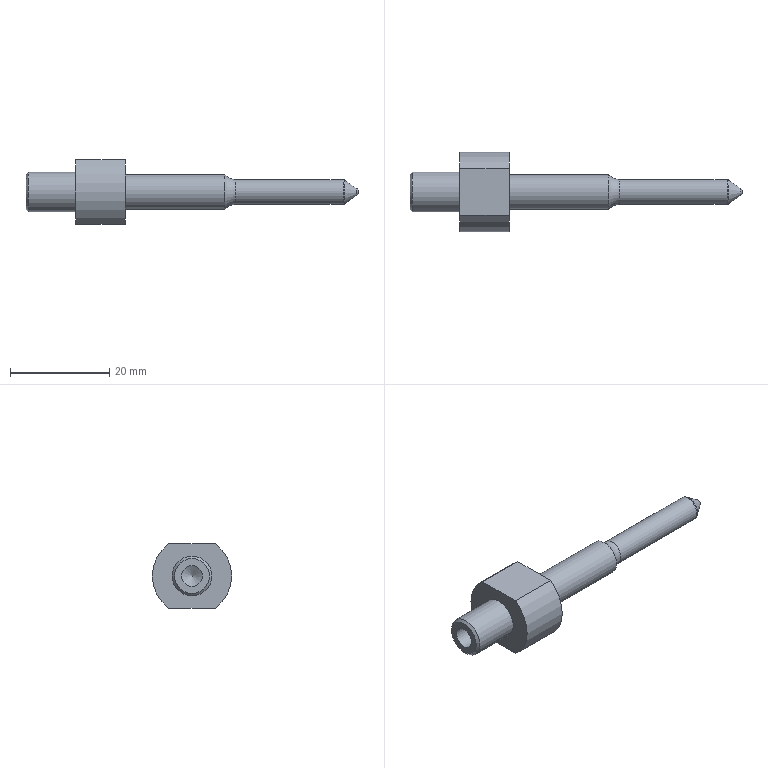Part | NX | features BREP 1 | 1 solid | 18 faces | box 66.856 x 16 x 13 mm | volume 3418 mm3 | cylinder 6 | plane 6 | torus 3 | cone 3 | commonest cylinder face diameters 16 x2 4.2 x1 5 x1 7 x1 8 x1
STEP:
#1=CARTESIAN_POINT('',(-13.428,0.,3.5));
#2=VERTEX_POINT('',#1);
#3=CARTESIAN_POINT('',(-13.428,0.,0.));
#4=DIRECTION('',(1.,0.,0.));
#5=DIRECTION('',(0.,0.,1.));
#6=AXIS2_PLACEMENT_3D('',#3,#4,#5);
#7=CIRCLE('',#6,3.5);
#8=EDGE_CURVE('',#2,#2,#7,.T.);
#9=ORIENTED_EDGE('',*,*,#8,.T.);
#10=EDGE_LOOP('',(#9));
#11=FACE_BOUND('',#10,.T.);
#12=CARTESIAN_POINT('',(6.572,0.,3.5));
#13=VERTEX_POINT('',#12);
#14=CARTESIAN_POINT('',(6.572,0.,0.));
#15=DIRECTION('',(-1.,0.,0.));
#16=DIRECTION('',(0.,0.,1.));
#17=AXIS2_PLACEMENT_3D('',#14,#15,#16);
#18=CIRCLE('',#17,3.5);
#19=EDGE_CURVE('',#13,#13,#18,.T.);
#20=ORIENTED_EDGE('',*,*,#19,.T.);
#21=EDGE_LOOP('',(#20));
#22=FACE_BOUND('',#21,.T.);
#23=CARTESIAN_POINT('',(6.572,0.,0.));
#24=DIRECTION('',(-1.,0.,0.));
#25=DIRECTION('',(0.,0.,-1.));
#26=AXIS2_PLACEMENT_3D('',#23,#24,#25);
#27=CYLINDRICAL_SURFACE('',#26,3.5);
#28=ADVANCED_FACE('',(#11,#22),#27,.T.);
#29=CARTESIAN_POINT('',(-13.428,4.664,-6.5));
#30=VERTEX_POINT('',#29);
#31=CARTESIAN_POINT('',(-13.428,-4.664,-6.5));
#32=VERTEX_POINT('',#31);
#33=CARTESIAN_POINT('',(-13.428,2.5,-6.5));
#34=DIRECTION('',(0.,-1.,0.));
#35=VECTOR('',#34,1000.);
#36=LINE('',#33,#35);
#37=EDGE_CURVE('',#30,#32,#36,.T.);
#38=ORIENTED_EDGE('',*,*,#37,.F.);
#39=CARTESIAN_POINT('',(-13.428,4.664,6.5));
#40=VERTEX_POINT('',#39);
#41=CARTESIAN_POINT('',(-13.428,0.,0.));
#42=DIRECTION('',(-1.,0.,0.));
#43=DIRECTION('',(0.,0.,1.));
#44=AXIS2_PLACEMENT_3D('',#41,#42,#43);
#45=CIRCLE('',#44,8.);
#46=EDGE_CURVE('',#40,#30,#45,.T.);
#47=ORIENTED_EDGE('',*,*,#46,.F.);
#48=CARTESIAN_POINT('',(-13.428,-4.664,6.5));
#49=VERTEX_POINT('',#48);
#50=CARTESIAN_POINT('',(-13.428,2.5,6.5));
#51=DIRECTION('',(0.,1.,0.));
#52=VECTOR('',#51,1000.);
#53=LINE('',#50,#52);
#54=EDGE_CURVE('',#49,#40,#53,.T.);
#55=ORIENTED_EDGE('',*,*,#54,.F.);
#56=CARTESIAN_POINT('',(-13.428,0.,0.));
#57=DIRECTION('',(-1.,0.,0.));
#58=DIRECTION('',(0.,0.,1.));
#59=AXIS2_PLACEMENT_3D('',#56,#57,#58);
#60=CIRCLE('',#59,8.);
#61=EDGE_CURVE('',#32,#49,#60,.T.);
#62=ORIENTED_EDGE('',*,*,#61,.F.);
#63=EDGE_LOOP('',(#38,#47,#55,#62));
#64=FACE_BOUND('',#63,.T.);
#65=ORIENTED_EDGE('',*,*,#8,.F.);
#66=EDGE_LOOP('',(#65));
#67=FACE_BOUND('',#66,.T.);
#68=CARTESIAN_POINT('',(-13.428,2.5,0.));
#69=DIRECTION('',(-1.,0.,0.));
#70=DIRECTION('',(0.,0.,-1.));
#71=AXIS2_PLACEMENT_3D('',#68,#69,#70);
#72=PLANE('',#71);
#73=ADVANCED_FACE('',(#64,#67),#72,.F.);
#74=ORIENTED_EDGE('',*,*,#19,.F.);
#75=EDGE_LOOP('',(#74));
#76=FACE_BOUND('',#75,.T.);
#77=CARTESIAN_POINT('',(8.808,0.,2.5));
#78=VERTEX_POINT('',#77);
#79=CARTESIAN_POINT('',(8.808,0.,0.));
#80=DIRECTION('',(1.,0.,0.));
#81=DIRECTION('',(0.,0.,1.));
#82=AXIS2_PLACEMENT_3D('',#79,#80,#81);
#83=CIRCLE('',#82,2.5);
#84=EDGE_CURVE('',#78,#78,#83,.T.);
#85=ORIENTED_EDGE('',*,*,#84,.F.);
#86=EDGE_LOOP('',(#85));
#87=FACE_BOUND('',#86,.T.);
#88=CARTESIAN_POINT('',(8.808,0.,0.));
#89=DIRECTION('',(-1.,0.,0.));
#90=DIRECTION('',(0.,0.,1.));
#91=AXIS2_PLACEMENT_3D('',#88,#89,#90);
#92=TOROIDAL_SURFACE('',#91,5.5,3.);
#93=ADVANCED_FACE('',(#76,#87),#92,.F.);
#94=ORIENTED_EDGE('',*,*,#61,.T.);
#95=CARTESIAN_POINT('',(-23.428,-4.664,6.5));
#96=VERTEX_POINT('',#95);
#97=CARTESIAN_POINT('',(-33.428,-4.664,6.5));
#98=DIRECTION('',(-1.,0.,0.));
#99=VECTOR('',#98,1000.);
#100=LINE('',#97,#99);
#101=EDGE_CURVE('',#49,#96,#100,.T.);
#102=ORIENTED_EDGE('',*,*,#101,.T.);
#103=CARTESIAN_POINT('',(-23.428,-4.664,-6.5));
#104=VERTEX_POINT('',#103);
#105=CARTESIAN_POINT('',(-23.428,0.,0.));
#106=DIRECTION('',(1.,0.,0.));
#107=DIRECTION('',(0.,0.,1.));
#108=AXIS2_PLACEMENT_3D('',#105,#106,#107);
#109=CIRCLE('',#108,8.);
#110=EDGE_CURVE('',#96,#104,#109,.T.);
#111=ORIENTED_EDGE('',*,*,#110,.T.);
#112=CARTESIAN_POINT('',(-33.428,-4.664,-6.5));
#113=DIRECTION('',(1.,0.,0.));
#114=VECTOR('',#113,1000.);
#115=LINE('',#112,#114);
#116=EDGE_CURVE('',#104,#32,#115,.T.);
#117=ORIENTED_EDGE('',*,*,#116,.T.);
#118=EDGE_LOOP('',(#94,#102,#111,#117));
#119=FACE_BOUND('',#118,.T.);
#120=CARTESIAN_POINT('',(-33.428,0.,0.));
#121=DIRECTION('',(-1.,0.,0.));
#122=DIRECTION('',(0.,0.,-1.));
#123=AXIS2_PLACEMENT_3D('',#120,#121,#122);
#124=CYLINDRICAL_SURFACE('',#123,8.);
#125=ADVANCED_FACE('',(#119),#124,.T.);
#126=ORIENTED_EDGE('',*,*,#116,.F.);
#127=CARTESIAN_POINT('',(-23.428,4.664,-6.5));
#128=VERTEX_POINT('',#127);
#129=CARTESIAN_POINT('',(-23.428,6.928,-6.5));
#130=DIRECTION('',(0.,-1.,0.));
#131=VECTOR('',#130,1000.);
#132=LINE('',#129,#131);
#133=EDGE_CURVE('',#128,#104,#132,.T.);
#134=ORIENTED_EDGE('',*,*,#133,.F.);
#135=CARTESIAN_POINT('',(33.428,4.664,-6.5));
#136=DIRECTION('',(-1.,0.,0.));
#137=VECTOR('',#136,1000.);
#138=LINE('',#135,#137);
#139=EDGE_CURVE('',#30,#128,#138,.T.);
#140=ORIENTED_EDGE('',*,*,#139,.F.);
#141=ORIENTED_EDGE('',*,*,#37,.T.);
#142=EDGE_LOOP('',(#126,#134,#140,#141));
#143=FACE_BOUND('',#142,.T.);
#144=CARTESIAN_POINT('',(33.428,6.928,-6.5));
#145=DIRECTION('',(0.,0.,1.));
#146=DIRECTION('',(-1.,0.,0.));
#147=AXIS2_PLACEMENT_3D('',#144,#145,#146);
#148=PLANE('',#147);
#149=ADVANCED_FACE('',(#143),#148,.F.);
#150=CARTESIAN_POINT('',(-23.428,4.664,6.5));
#151=VERTEX_POINT('',#150);
#152=CARTESIAN_POINT('',(-23.428,0.,0.));
#153=DIRECTION('',(1.,0.,0.));
#154=DIRECTION('',(0.,0.,1.));
#155=AXIS2_PLACEMENT_3D('',#152,#153,#154);
#156=CIRCLE('',#155,8.);
#157=EDGE_CURVE('',#128,#151,#156,.T.);
#158=ORIENTED_EDGE('',*,*,#157,.T.);
#159=CARTESIAN_POINT('',(-33.428,4.664,6.5));
#160=DIRECTION('',(1.,0.,0.));
#161=VECTOR('',#160,1000.);
#162=LINE('',#159,#161);
#163=EDGE_CURVE('',#151,#40,#162,.T.);
#164=ORIENTED_EDGE('',*,*,#163,.T.);
#165=ORIENTED_EDGE('',*,*,#46,.T.);
#166=ORIENTED_EDGE('',*,*,#139,.T.);
#167=EDGE_LOOP('',(#158,#164,#165,#166));
#168=FACE_BOUND('',#167,.T.);
#169=CARTESIAN_POINT('',(-33.428,0.,0.));
#170=DIRECTION('',(-1.,0.,0.));
#171=DIRECTION('',(0.,0.,-1.));
#172=AXIS2_PLACEMENT_3D('',#169,#170,#171);
#173=CYLINDRICAL_SURFACE('',#172,8.);
#174=ADVANCED_FACE('',(#168),#173,.T.);
#175=ORIENTED_EDGE('',*,*,#163,.F.);
#176=CARTESIAN_POINT('',(-23.428,7.156,6.5));
#177=DIRECTION('',(0.,1.,0.));
#178=VECTOR('',#177,1000.);
#179=LINE('',#176,#178);
#180=EDGE_CURVE('',#96,#151,#179,.T.);
#181=ORIENTED_EDGE('',*,*,#180,.F.);
#182=ORIENTED_EDGE('',*,*,#101,.F.);
#183=ORIENTED_EDGE('',*,*,#54,.T.);
#184=EDGE_LOOP('',(#175,#181,#182,#183));
#185=FACE_BOUND('',#184,.T.);
#186=CARTESIAN_POINT('',(33.428,7.156,6.5));
#187=DIRECTION('',(0.,0.,-1.));
#188=DIRECTION('',(1.,0.,0.));
#189=AXIS2_PLACEMENT_3D('',#186,#187,#188);
#190=PLANE('',#189);
#191=ADVANCED_FACE('',(#185),#190,.F.);
#192=ORIENTED_EDGE('',*,*,#84,.T.);
#193=EDGE_LOOP('',(#192));
#194=FACE_BOUND('',#193,.T.);
#195=CARTESIAN_POINT('',(30.414,0.,2.5));
#196=VERTEX_POINT('',#195);
#197=CARTESIAN_POINT('',(30.414,0.,0.));
#198=DIRECTION('',(-1.,0.,0.));
#199=DIRECTION('',(0.,0.,1.));
#200=AXIS2_PLACEMENT_3D('',#197,#198,#199);
#201=CIRCLE('',#200,2.5);
#202=EDGE_CURVE('',#196,#196,#201,.T.);
#203=ORIENTED_EDGE('',*,*,#202,.T.);
#204=EDGE_LOOP('',(#203));
#205=FACE_BOUND('',#204,.T.);
#206=CARTESIAN_POINT('',(-33.428,0.,0.));
#207=DIRECTION('',(-1.,0.,0.));
#208=DIRECTION('',(0.,0.,-1.));
#209=AXIS2_PLACEMENT_3D('',#206,#207,#208);
#210=CYLINDRICAL_SURFACE('',#209,2.5);
#211=ADVANCED_FACE('',(#194,#205),#210,.T.);
#212=ORIENTED_EDGE('',*,*,#133,.T.);
#213=ORIENTED_EDGE('',*,*,#110,.F.);
#214=ORIENTED_EDGE('',*,*,#180,.T.);
#215=ORIENTED_EDGE('',*,*,#157,.F.);
#216=EDGE_LOOP('',(#212,#213,#214,#215));
#217=FACE_BOUND('',#216,.T.);
#218=CARTESIAN_POINT('',(-23.428,0.,4.));
#219=VERTEX_POINT('',#218);
#220=CARTESIAN_POINT('',(-23.428,0.,0.));
#221=DIRECTION('',(-1.,0.,0.));
#222=DIRECTION('',(0.,0.,1.));
#223=AXIS2_PLACEMENT_3D('',#220,#221,#222);
#224=CIRCLE('',#223,4.);
#225=EDGE_CURVE('',#219,#219,#224,.T.);
#226=ORIENTED_EDGE('',*,*,#225,.F.);
#227=EDGE_LOOP('',(#226));
#228=FACE_BOUND('',#227,.T.);
#229=CARTESIAN_POINT('',(-23.428,8.,0.));
#230=DIRECTION('',(1.,0.,0.));
#231=DIRECTION('',(0.,0.,1.));
#232=AXIS2_PLACEMENT_3D('',#229,#230,#231);
#233=PLANE('',#232);
#234=ADVANCED_FACE('',(#217,#228),#233,.F.);
#235=CARTESIAN_POINT('',(30.701,0.,-2.41));
#236=VERTEX_POINT('',#235);
#237=CARTESIAN_POINT('',(30.701,0.,0.));
#238=DIRECTION('',(-1.,0.,0.));
#239=DIRECTION('',(0.,0.,-1.));
#240=AXIS2_PLACEMENT_3D('',#237,#238,#239);
#241=CIRCLE('',#240,2.41);
#242=EDGE_CURVE('',#236,#236,#241,.T.);
#243=ORIENTED_EDGE('',*,*,#242,.T.);
#244=EDGE_LOOP('',(#243));
#245=FACE_BOUND('',#244,.T.);
#246=ORIENTED_EDGE('',*,*,#202,.F.);
#247=EDGE_LOOP('',(#246));
#248=FACE_BOUND('',#247,.T.);
#249=CARTESIAN_POINT('',(30.414,0.,0.));
#250=DIRECTION('',(1.,0.,0.));
#251=DIRECTION('',(0.,0.,-1.));
#252=AXIS2_PLACEMENT_3D('',#249,#250,#251);
#253=TOROIDAL_SURFACE('',#252,2.,0.5);
#254=ADVANCED_FACE('',(#245,#248),#253,.T.);
#255=CARTESIAN_POINT('',(-32.928,0.,4.));
#256=VERTEX_POINT('',#255);
#257=CARTESIAN_POINT('',(-32.928,0.,0.));
#258=DIRECTION('',(1.,0.,0.));
#259=DIRECTION('',(0.,0.,1.));
#260=AXIS2_PLACEMENT_3D('',#257,#258,#259);
#261=CIRCLE('',#260,4.);
#262=EDGE_CURVE('',#256,#256,#261,.T.);
#263=ORIENTED_EDGE('',*,*,#262,.T.);
#264=EDGE_LOOP('',(#263));
#265=FACE_BOUND('',#264,.T.);
#266=ORIENTED_EDGE('',*,*,#225,.T.);
#267=EDGE_LOOP('',(#266));
#268=FACE_BOUND('',#267,.T.);
#269=CARTESIAN_POINT('',(-33.428,0.,0.));
#270=DIRECTION('',(-1.,0.,0.));
#271=DIRECTION('',(0.,0.,-1.));
#272=AXIS2_PLACEMENT_3D('',#269,#270,#271);
#273=CYLINDRICAL_SURFACE('',#272,4.);
#274=ADVANCED_FACE('',(#265,#268),#273,.T.);
#275=ORIENTED_EDGE('',*,*,#242,.F.);
#276=EDGE_LOOP('',(#275));
#277=FACE_BOUND('',#276,.T.);
#278=CARTESIAN_POINT('',(33.215,0.,0.6493));
#279=VERTEX_POINT('',#278);
#280=CARTESIAN_POINT('',(33.215,0.,0.));
#281=DIRECTION('',(-1.,0.,0.));
#282=DIRECTION('',(0.,0.,1.));
#283=AXIS2_PLACEMENT_3D('',#280,#281,#282);
#284=CIRCLE('',#283,0.6493);
#285=EDGE_CURVE('',#279,#279,#284,.T.);
#286=ORIENTED_EDGE('',*,*,#285,.T.);
#287=EDGE_LOOP('',(#286));
#288=FACE_BOUND('',#287,.T.);
#289=CARTESIAN_POINT('',(30.701,0.,0.));
#290=DIRECTION('',(-1.,0.,0.));
#291=DIRECTION('',(0.,0.,-1.));
#292=AXIS2_PLACEMENT_3D('',#289,#290,#291);
#293=CONICAL_SURFACE('',#292,2.41,0.6109);
#294=ADVANCED_FACE('',(#277,#288),#293,.T.);
#295=ORIENTED_EDGE('',*,*,#262,.F.);
#296=EDGE_LOOP('',(#295));
#297=FACE_BOUND('',#296,.T.);
#298=CARTESIAN_POINT('',(-33.428,0.,-3.5));
#299=VERTEX_POINT('',#298);
#300=CARTESIAN_POINT('',(-33.428,0.,0.));
#301=DIRECTION('',(1.,0.,0.));
#302=DIRECTION('',(0.,0.,-1.));
#303=AXIS2_PLACEMENT_3D('',#300,#301,#302);
#304=CIRCLE('',#303,3.5);
#305=EDGE_CURVE('',#299,#299,#304,.T.);
#306=ORIENTED_EDGE('',*,*,#305,.T.);
#307=EDGE_LOOP('',(#306));
#308=FACE_BOUND('',#307,.T.);
#309=CARTESIAN_POINT('',(-32.928,0.,0.));
#310=DIRECTION('',(1.,0.,0.));
#311=DIRECTION('',(0.,0.,1.));
#312=AXIS2_PLACEMENT_3D('',#309,#310,#311);
#313=CONICAL_SURFACE('',#312,4.,0.7854);
#314=ADVANCED_FACE('',(#297,#308),#313,.T.);
#315=ORIENTED_EDGE('',*,*,#285,.F.);
#316=EDGE_LOOP('',(#315));
#317=FACE_BOUND('',#316,.T.);
#318=CARTESIAN_POINT('',(33.428,0.,0.2397));
#319=VERTEX_POINT('',#318);
#320=CARTESIAN_POINT('',(33.428,0.,-0.2397));
#321=VERTEX_POINT('',#320);
#322=CARTESIAN_POINT('',(33.428,0.,0.));
#323=DIRECTION('',(-1.,0.,0.));
#324=DIRECTION('',(0.,0.,1.));
#325=AXIS2_PLACEMENT_3D('',#322,#323,#324);
#326=CIRCLE('',#325,0.2397);
#327=EDGE_CURVE('',#319,#321,#326,.T.);
#328=ORIENTED_EDGE('',*,*,#327,.T.);
#329=CARTESIAN_POINT('',(33.428,0.,0.));
#330=DIRECTION('',(-1.,0.,0.));
#331=DIRECTION('',(0.,0.,1.));
#332=AXIS2_PLACEMENT_3D('',#329,#330,#331);
#333=CIRCLE('',#332,0.2397);
#334=EDGE_CURVE('',#321,#319,#333,.T.);
#335=ORIENTED_EDGE('',*,*,#334,.T.);
#336=EDGE_LOOP('',(#328,#335));
#337=FACE_BOUND('',#336,.T.);
#338=CARTESIAN_POINT('',(32.928,0.,0.));
#339=DIRECTION('',(-1.,0.,0.));
#340=DIRECTION('',(0.,0.,1.));
#341=AXIS2_PLACEMENT_3D('',#338,#339,#340);
#342=DEGENERATE_TOROIDAL_SURFACE('',#341,0.2397,0.5,.T.);
#343=ADVANCED_FACE('',(#317,#337),#342,.T.);
#344=CARTESIAN_POINT('',(-33.428,0.,2.1));
#345=VERTEX_POINT('',#344);
#346=CARTESIAN_POINT('',(-33.428,0.,0.));
#347=DIRECTION('',(-1.,0.,0.));
#348=DIRECTION('',(0.,0.,1.));
#349=AXIS2_PLACEMENT_3D('',#346,#347,#348);
#350=CIRCLE('',#349,2.1);
#351=EDGE_CURVE('',#345,#345,#350,.T.);
#352=ORIENTED_EDGE('',*,*,#351,.F.);
#353=EDGE_LOOP('',(#352));
#354=FACE_BOUND('',#353,.T.);
#355=ORIENTED_EDGE('',*,*,#305,.F.);
#356=EDGE_LOOP('',(#355));
#357=FACE_BOUND('',#356,.T.);
#358=CARTESIAN_POINT('',(-33.428,4.,0.));
#359=DIRECTION('',(1.,0.,0.));
#360=DIRECTION('',(0.,0.,1.));
#361=AXIS2_PLACEMENT_3D('',#358,#359,#360);
#362=PLANE('',#361);
#363=ADVANCED_FACE('',(#354,#357),#362,.F.);
#364=ORIENTED_EDGE('',*,*,#327,.F.);
#365=ORIENTED_EDGE('',*,*,#334,.F.);
#366=EDGE_LOOP('',(#364,#365));
#367=FACE_BOUND('',#366,.T.);
#368=CARTESIAN_POINT('',(33.428,0.,0.));
#369=DIRECTION('',(-1.,0.,0.));
#370=DIRECTION('',(0.,0.,-1.));
#371=AXIS2_PLACEMENT_3D('',#368,#369,#370);
#372=PLANE('',#371);
#373=ADVANCED_FACE('',(#367),#372,.F.);
#374=CARTESIAN_POINT('',(-21.028,0.,2.1));
#375=VERTEX_POINT('',#374);
#376=CARTESIAN_POINT('',(-21.028,0.,0.));
#377=DIRECTION('',(-1.,0.,0.));
#378=DIRECTION('',(0.,0.,1.));
#379=AXIS2_PLACEMENT_3D('',#376,#377,#378);
#380=CIRCLE('',#379,2.1);
#381=EDGE_CURVE('',#375,#375,#380,.T.);
#382=ORIENTED_EDGE('',*,*,#381,.F.);
#383=EDGE_LOOP('',(#382));
#384=FACE_BOUND('',#383,.T.);
#385=ORIENTED_EDGE('',*,*,#351,.T.);
#386=EDGE_LOOP('',(#385));
#387=FACE_BOUND('',#386,.T.);
#388=CARTESIAN_POINT('',(-33.428,0.,0.));
#389=DIRECTION('',(-1.,0.,0.));
#390=DIRECTION('',(0.,0.,-1.));
#391=AXIS2_PLACEMENT_3D('',#388,#389,#390);
#392=CYLINDRICAL_SURFACE('',#391,2.1);
#393=ADVANCED_FACE('',(#384,#387),#392,.F.);
#394=CARTESIAN_POINT('',(-19.766,0.,0.));
#395=VERTEX_POINT('',#394);
#396=VERTEX_LOOP('',#395);
#397=FACE_BOUND('',#396,.T.);
#398=ORIENTED_EDGE('',*,*,#381,.T.);
#399=EDGE_LOOP('',(#398));
#400=FACE_BOUND('',#399,.T.);
#401=CARTESIAN_POINT('',(-21.028,0.,0.));
#402=DIRECTION('',(-1.,0.,0.));
#403=DIRECTION('',(0.,0.,-1.));
#404=AXIS2_PLACEMENT_3D('',#401,#402,#403);
#405=CONICAL_SURFACE('',#404,2.1,1.03);
#406=ADVANCED_FACE('',(#397,#400),#405,.F.);
#407=CLOSED_SHELL('',(#28,#73,#93,#125,#149,#174,#191,#211,#234,#254,#274,#294,#314,#343,#363,#373,#393,#406));
#408=MANIFOLD_SOLID_BREP('',#407);
#409=(LENGTH_UNIT()NAMED_UNIT(*)SI_UNIT(.MILLI.,.METRE.));
#410=UNCERTAINTY_MEASURE_WITH_UNIT(LENGTH_MEASURE(0.00001),#409,'','');
#411=(NAMED_UNIT(*)PLANE_ANGLE_UNIT()SI_UNIT($,.RADIAN.));
#412=(NAMED_UNIT(*)SI_UNIT($,.STERADIAN.)SOLID_ANGLE_UNIT());
#413=(GEOMETRIC_REPRESENTATION_CONTEXT(3)GLOBAL_UNCERTAINTY_ASSIGNED_CONTEXT((#410))GLOBAL_UNIT_ASSIGNED_CONTEXT((#409,#411,#412))REPRESENTATION_CONTEXT('',''));
#414=ADVANCED_BREP_SHAPE_REPRESENTATION('',(#408),#413);